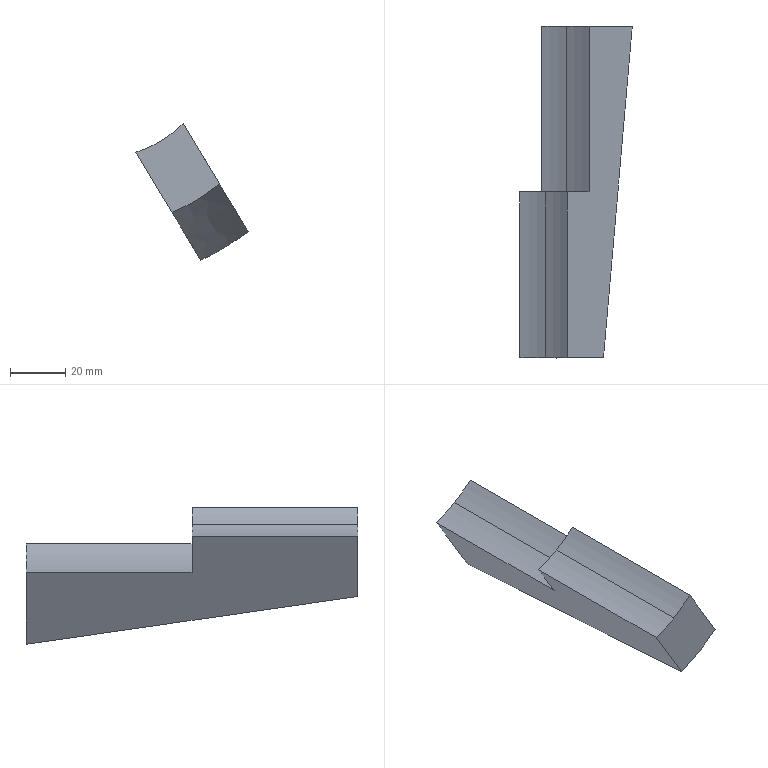Part | STEP file | 2026.6.15-Main Assembly图.sldasm-Part-37 | 1 solid | 10 faces | box 40.625 x 120 x 49.357 mm | volume 66279 mm3 | plane 5 | cylinder 4 | spline 1 | commonest cylinder face diameters 90 x2 120 x2
STEP:
#1=CARTESIAN_POINT('',(-731.198,648.541,3155.98));
#2=VERTEX_POINT('',#1);
#3=CARTESIAN_POINT('',(-740.348,648.541,3151.791));
#4=VERTEX_POINT('',#3);
#5=CARTESIAN_POINT('',(-754.391,648.541,3194.543));
#6=DIRECTION('',(0.,1.,0.));
#7=DIRECTION('',(0.5154,0.,-0.8569));
#8=AXIS2_PLACEMENT_3D('',#5,#6,#7);
#9=CIRCLE('',#8,45.);
#10=EDGE_CURVE('',#2,#4,#9,.T.);
#11=ORIENTED_EDGE('',*,*,#10,.F.);
#12=CARTESIAN_POINT('',(-731.198,708.541,3155.98));
#13=VERTEX_POINT('',#12);
#14=CARTESIAN_POINT('',(-731.198,648.541,3155.98));
#15=DIRECTION('',(0.,1.,0.));
#16=VECTOR('',#15,1000.);
#17=LINE('',#14,#16);
#18=EDGE_CURVE('',#2,#13,#17,.T.);
#19=ORIENTED_EDGE('',*,*,#18,.T.);
#20=CARTESIAN_POINT('',(-740.348,708.541,3151.791));
#21=VERTEX_POINT('',#20);
#22=CARTESIAN_POINT('',(-754.391,708.541,3194.543));
#23=DIRECTION('',(0.,-1.,0.));
#24=DIRECTION('',(0.5154,0.,-0.8569));
#25=AXIS2_PLACEMENT_3D('',#22,#23,#24);
#26=CIRCLE('',#25,45.);
#27=EDGE_CURVE('',#21,#13,#26,.T.);
#28=ORIENTED_EDGE('',*,*,#27,.F.);
#29=CARTESIAN_POINT('',(-740.348,648.541,3151.791));
#30=DIRECTION('',(0.,-1.,0.));
#31=VECTOR('',#30,1000.);
#32=LINE('',#29,#31);
#33=EDGE_CURVE('',#21,#4,#32,.T.);
#34=ORIENTED_EDGE('',*,*,#33,.T.);
#35=EDGE_LOOP('',(#11,#19,#28,#34));
#36=FACE_OUTER_BOUND('',#35,.T.);
#37=CARTESIAN_POINT('',(-754.391,648.541,3194.543));
#38=DIRECTION('',(0.,1.,0.));
#39=DIRECTION('',(-0.5154,0.,0.8569));
#40=AXIS2_PLACEMENT_3D('',#37,#38,#39);
#41=CYLINDRICAL_SURFACE('',#40,45.);
#42=ADVANCED_FACE('',(#36),#41,.F.);
#43=CARTESIAN_POINT('',(-723.467,708.541,3143.126));
#44=VERTEX_POINT('',#43);
#45=CARTESIAN_POINT('',(-732.469,708.541,3138.691));
#46=VERTEX_POINT('',#45);
#47=CARTESIAN_POINT('',(-754.391,708.541,3194.543));
#48=DIRECTION('',(0.,1.,0.));
#49=DIRECTION('',(0.5154,0.,-0.8569));
#50=AXIS2_PLACEMENT_3D('',#47,#48,#49);
#51=CIRCLE('',#50,60.);
#52=EDGE_CURVE('',#44,#46,#51,.T.);
#53=ORIENTED_EDGE('',*,*,#52,.F.);
#54=CARTESIAN_POINT('',(-723.467,768.541,3143.126));
#55=VERTEX_POINT('',#54);
#56=CARTESIAN_POINT('',(-723.467,708.541,3143.126));
#57=DIRECTION('',(0.,1.,0.));
#58=VECTOR('',#57,1000.);
#59=LINE('',#56,#58);
#60=EDGE_CURVE('',#44,#55,#59,.T.);
#61=ORIENTED_EDGE('',*,*,#60,.T.);
#62=CARTESIAN_POINT('',(-732.469,768.541,3138.691));
#63=VERTEX_POINT('',#62);
#64=CARTESIAN_POINT('',(-754.391,768.541,3194.543));
#65=DIRECTION('',(0.,1.,0.));
#66=DIRECTION('',(0.5154,0.,-0.8569));
#67=AXIS2_PLACEMENT_3D('',#64,#65,#66);
#68=CIRCLE('',#67,60.);
#69=EDGE_CURVE('',#55,#63,#68,.T.);
#70=ORIENTED_EDGE('',*,*,#69,.T.);
#71=CARTESIAN_POINT('',(-732.469,708.541,3138.691));
#72=DIRECTION('',(0.,-1.,0.));
#73=VECTOR('',#72,1000.);
#74=LINE('',#71,#73);
#75=EDGE_CURVE('',#63,#46,#74,.T.);
#76=ORIENTED_EDGE('',*,*,#75,.T.);
#77=EDGE_LOOP('',(#53,#61,#70,#76));
#78=FACE_OUTER_BOUND('',#77,.T.);
#79=CARTESIAN_POINT('',(-754.391,708.541,3194.543));
#80=DIRECTION('',(0.,1.,0.));
#81=DIRECTION('',(-0.5154,0.,0.8569));
#82=AXIS2_PLACEMENT_3D('',#79,#80,#81);
#83=CYLINDRICAL_SURFACE('',#82,60.);
#84=ADVANCED_FACE('',(#78),#83,.F.);
#85=ORIENTED_EDGE('',*,*,#60,.F.);
#86=CARTESIAN_POINT('',(-715.33,708.541,3148.999));
#87=VERTEX_POINT('',#86);
#88=CARTESIAN_POINT('',(-754.391,708.541,3194.543));
#89=DIRECTION('',(0.,1.,0.));
#90=DIRECTION('',(0.5154,0.,-0.8569));
#91=AXIS2_PLACEMENT_3D('',#88,#89,#90);
#92=CIRCLE('',#91,60.);
#93=EDGE_CURVE('',#87,#44,#92,.T.);
#94=ORIENTED_EDGE('',*,*,#93,.F.);
#95=CARTESIAN_POINT('',(-715.33,768.541,3148.999));
#96=VERTEX_POINT('',#95);
#97=CARTESIAN_POINT('',(-715.33,708.541,3148.999));
#98=DIRECTION('',(0.,1.,0.));
#99=VECTOR('',#98,1000.);
#100=LINE('',#97,#99);
#101=EDGE_CURVE('',#87,#96,#100,.T.);
#102=ORIENTED_EDGE('',*,*,#101,.T.);
#103=CARTESIAN_POINT('',(-754.391,768.541,3194.543));
#104=DIRECTION('',(0.,1.,0.));
#105=DIRECTION('',(0.5154,0.,-0.8569));
#106=AXIS2_PLACEMENT_3D('',#103,#104,#105);
#107=CIRCLE('',#106,60.);
#108=EDGE_CURVE('',#96,#55,#107,.T.);
#109=ORIENTED_EDGE('',*,*,#108,.T.);
#110=EDGE_LOOP('',(#85,#94,#102,#109));
#111=FACE_OUTER_BOUND('',#110,.T.);
#112=CARTESIAN_POINT('',(-754.391,708.541,3194.543));
#113=DIRECTION('',(0.,1.,0.));
#114=DIRECTION('',(-0.5154,0.,0.8569));
#115=AXIS2_PLACEMENT_3D('',#112,#113,#114);
#116=CYLINDRICAL_SURFACE('',#115,60.);
#117=ADVANCED_FACE('',(#111),#116,.F.);
#118=CARTESIAN_POINT('',(-723.209,708.541,3162.099));
#119=VERTEX_POINT('',#118);
#120=CARTESIAN_POINT('',(-745.822,708.541,3199.697));
#121=DIRECTION('',(-0.5154,0.,0.8569));
#122=VECTOR('',#121,1000.);
#123=LINE('',#120,#122);
#124=EDGE_CURVE('',#87,#119,#123,.T.);
#125=ORIENTED_EDGE('',*,*,#124,.F.);
#126=ORIENTED_EDGE('',*,*,#93,.T.);
#127=ORIENTED_EDGE('',*,*,#52,.T.);
#128=CARTESIAN_POINT('',(-762.961,708.541,3189.389));
#129=DIRECTION('',(0.5154,0.,-0.8569));
#130=VECTOR('',#129,1000.);
#131=LINE('',#128,#130);
#132=EDGE_CURVE('',#21,#46,#131,.T.);
#133=ORIENTED_EDGE('',*,*,#132,.F.);
#134=ORIENTED_EDGE('',*,*,#27,.T.);
#135=CARTESIAN_POINT('',(-754.391,708.541,3194.543));
#136=DIRECTION('',(0.,-1.,0.));
#137=DIRECTION('',(0.5154,0.,-0.8569));
#138=AXIS2_PLACEMENT_3D('',#135,#136,#137);
#139=CIRCLE('',#138,45.);
#140=EDGE_CURVE('',#13,#119,#139,.T.);
#141=ORIENTED_EDGE('',*,*,#140,.T.);
#142=EDGE_LOOP('',(#125,#126,#127,#133,#134,#141));
#143=FACE_OUTER_BOUND('',#142,.T.);
#144=CARTESIAN_POINT('',(-754.391,708.541,3194.543));
#145=DIRECTION('',(0.,1.,0.));
#146=DIRECTION('',(0.8569,0.,0.5154));
#147=AXIS2_PLACEMENT_3D('',#144,#145,#146);
#148=PLANE('',#147);
#149=ADVANCED_FACE('',(#143),#148,.T.);
#150=CARTESIAN_POINT('',(-710.114,648.541,3140.326));
#151=VERTEX_POINT('',#150);
#152=CARTESIAN_POINT('',(-699.723,768.541,3123.049));
#153=VERTEX_POINT('',#152);
#154=CARTESIAN_POINT('',(-710.114,648.541,3140.326));
#155=CARTESIAN_POINT('',(-709.101,660.212,3138.642));
#156=CARTESIAN_POINT('',(-708.089,671.882,3136.959));
#157=CARTESIAN_POINT('',(-707.077,683.553,3135.278));
#158=CARTESIAN_POINT('',(-706.066,695.224,3133.596));
#159=CARTESIAN_POINT('',(-705.055,706.895,3131.916));
#160=CARTESIAN_POINT('',(-704.045,718.566,3130.236));
#161=CARTESIAN_POINT('',(-702.603,735.224,3127.839));
#162=CARTESIAN_POINT('',(-701.163,751.882,3125.443));
#163=CARTESIAN_POINT('',(-699.723,768.541,3123.049));
#164=B_SPLINE_CURVE_WITH_KNOTS('',3,(#154,#155,#156,#157,#158,#159,#160,#161,#162,#163),.UNSPECIFIED.,.F.,.F.,(4,3,3,4),(0.,0.0355,0.07101,0.1217),.UNSPECIFIED.);
#165=EDGE_CURVE('',#151,#153,#164,.T.);
#166=ORIENTED_EDGE('',*,*,#165,.F.);
#167=CARTESIAN_POINT('',(-727.253,648.541,3130.018));
#168=VERTEX_POINT('',#167);
#169=CARTESIAN_POINT('',(-710.114,648.541,3140.326));
#170=CARTESIAN_POINT('',(-712.704,648.541,3138.21));
#171=CARTESIAN_POINT('',(-718.189,648.541,3134.35));
#172=CARTESIAN_POINT('',(-724.17,648.541,3131.315));
#173=CARTESIAN_POINT('',(-727.253,648.541,3130.018));
#174=B_SPLINE_CURVE_WITH_KNOTS('',3,(#169,#170,#171,#172,#173),.UNSPECIFIED.,.F.,.F.,(4,1,4),(0.,0.01,0.02),.UNSPECIFIED.);
#175=EDGE_CURVE('',#151,#168,#174,.T.);
#176=ORIENTED_EDGE('',*,*,#175,.T.);
#177=CARTESIAN_POINT('',(-716.862,768.541,3112.741));
#178=VERTEX_POINT('',#177);
#179=CARTESIAN_POINT('',(-716.862,768.541,3112.741));
#180=CARTESIAN_POINT('',(-717.925,756.246,3114.508));
#181=CARTESIAN_POINT('',(-718.988,743.952,3116.276));
#182=CARTESIAN_POINT('',(-720.051,731.657,3118.045));
#183=CARTESIAN_POINT('',(-721.115,719.363,3119.813));
#184=CARTESIAN_POINT('',(-722.179,707.068,3121.583));
#185=CARTESIAN_POINT('',(-723.244,694.774,3123.353));
#186=CARTESIAN_POINT('',(-724.579,679.363,3125.573));
#187=CARTESIAN_POINT('',(-725.915,663.952,3127.794));
#188=CARTESIAN_POINT('',(-727.253,648.541,3130.018));
#189=B_SPLINE_CURVE_WITH_KNOTS('',3,(#179,#180,#181,#182,#183,#184,#185,#186,#187,#188),.UNSPECIFIED.,.F.,.F.,(4,3,3,4),(0.,0.0374,0.0748,0.1217),.UNSPECIFIED.);
#190=EDGE_CURVE('',#178,#168,#189,.T.);
#191=ORIENTED_EDGE('',*,*,#190,.F.);
#192=CARTESIAN_POINT('',(-699.723,768.541,3123.049));
#193=CARTESIAN_POINT('',(-702.376,768.541,3121.02));
#194=CARTESIAN_POINT('',(-707.909,768.541,3117.258));
#195=CARTESIAN_POINT('',(-713.826,768.541,3114.134));
#196=CARTESIAN_POINT('',(-716.862,768.541,3112.741));
#197=B_SPLINE_CURVE_WITH_KNOTS('',3,(#192,#193,#194,#195,#196),.UNSPECIFIED.,.F.,.F.,(4,1,4),(0.,0.01,0.02),.UNSPECIFIED.);
#198=EDGE_CURVE('',#153,#178,#197,.T.);
#199=ORIENTED_EDGE('',*,*,#198,.F.);
#200=EDGE_LOOP('',(#166,#176,#191,#199));
#201=FACE_OUTER_BOUND('',#200,.T.);
#202=CARTESIAN_POINT('',(-677.094,769.741,3241.032));
#203=CARTESIAN_POINT('',(-677.152,769.341,3240.998));
#204=CARTESIAN_POINT('',(-677.209,768.941,3240.964));
#205=CARTESIAN_POINT('',(-677.266,768.541,3240.929));
#206=CARTESIAN_POINT('',(-682.979,728.541,3237.493));
#207=CARTESIAN_POINT('',(-688.692,688.541,3234.057));
#208=CARTESIAN_POINT('',(-694.405,648.541,3230.621));
#209=CARTESIAN_POINT('',(-680.137,769.741,3246.091));
#210=CARTESIAN_POINT('',(-680.192,769.341,3246.053));
#211=CARTESIAN_POINT('',(-680.247,768.941,3246.015));
#212=CARTESIAN_POINT('',(-680.302,768.541,3245.977));
#213=CARTESIAN_POINT('',(-685.79,728.541,3242.167));
#214=CARTESIAN_POINT('',(-691.278,688.541,3238.357));
#215=CARTESIAN_POINT('',(-696.766,648.541,3234.547));
#216=CARTESIAN_POINT('',(-687.219,769.741,3255.61));
#217=CARTESIAN_POINT('',(-687.268,769.341,3255.565));
#218=CARTESIAN_POINT('',(-687.318,768.941,3255.52));
#219=CARTESIAN_POINT('',(-687.368,768.541,3255.475));
#220=CARTESIAN_POINT('',(-692.332,728.541,3250.961));
#221=CARTESIAN_POINT('',(-697.297,688.541,3246.448));
#222=CARTESIAN_POINT('',(-702.262,648.541,3241.934));
#223=CARTESIAN_POINT('',(-700.423,769.741,3267.541));
#224=CARTESIAN_POINT('',(-700.463,769.341,3267.487));
#225=CARTESIAN_POINT('',(-700.503,768.941,3267.433));
#226=CARTESIAN_POINT('',(-700.543,768.541,3267.379));
#227=CARTESIAN_POINT('',(-704.532,728.541,3261.984));
#228=CARTESIAN_POINT('',(-708.52,688.541,3256.589));
#229=CARTESIAN_POINT('',(-712.509,648.541,3251.194));
#230=CARTESIAN_POINT('',(-715.701,769.741,3276.667));
#231=CARTESIAN_POINT('',(-715.73,769.341,3276.607));
#232=CARTESIAN_POINT('',(-715.759,768.941,3276.546));
#233=CARTESIAN_POINT('',(-715.787,768.541,3276.485));
#234=CARTESIAN_POINT('',(-718.647,728.541,3270.415));
#235=CARTESIAN_POINT('',(-721.506,688.541,3264.346));
#236=CARTESIAN_POINT('',(-724.366,648.541,3258.276));
#237=CARTESIAN_POINT('',(-732.467,769.741,3282.637));
#238=CARTESIAN_POINT('',(-732.483,769.341,3282.572));
#239=CARTESIAN_POINT('',(-732.499,768.941,3282.507));
#240=CARTESIAN_POINT('',(-732.515,768.541,3282.442));
#241=CARTESIAN_POINT('',(-734.136,728.541,3275.931));
#242=CARTESIAN_POINT('',(-735.756,688.541,3269.42));
#243=CARTESIAN_POINT('',(-737.376,648.541,3262.909));
#244=CARTESIAN_POINT('',(-750.074,769.741,3285.222));
#245=CARTESIAN_POINT('',(-750.077,769.341,3285.155));
#246=CARTESIAN_POINT('',(-750.08,768.941,3285.088));
#247=CARTESIAN_POINT('',(-750.084,768.541,3285.021));
#248=CARTESIAN_POINT('',(-750.403,728.541,3278.319));
#249=CARTESIAN_POINT('',(-750.722,688.541,3271.617));
#250=CARTESIAN_POINT('',(-751.041,648.541,3264.915));
#251=CARTESIAN_POINT('',(-767.848,769.741,3284.322));
#252=CARTESIAN_POINT('',(-767.838,769.341,3284.255));
#253=CARTESIAN_POINT('',(-767.828,768.941,3284.189));
#254=CARTESIAN_POINT('',(-767.818,768.541,3284.123));
#255=CARTESIAN_POINT('',(-766.823,728.541,3277.487));
#256=CARTESIAN_POINT('',(-765.829,688.541,3270.852));
#257=CARTESIAN_POINT('',(-764.834,648.541,3264.216));
#258=CARTESIAN_POINT('',(-785.104,769.741,3279.971));
#259=CARTESIAN_POINT('',(-785.081,769.341,3279.908));
#260=CARTESIAN_POINT('',(-785.059,768.941,3279.845));
#261=CARTESIAN_POINT('',(-785.036,768.541,3279.782));
#262=CARTESIAN_POINT('',(-782.766,728.541,3273.468));
#263=CARTESIAN_POINT('',(-780.496,688.541,3267.154));
#264=CARTESIAN_POINT('',(-778.226,648.541,3260.84));
#265=CARTESIAN_POINT('',(-801.18,769.741,3272.338));
#266=CARTESIAN_POINT('',(-801.146,769.341,3272.281));
#267=CARTESIAN_POINT('',(-801.111,768.941,3272.223));
#268=CARTESIAN_POINT('',(-801.076,768.541,3272.166));
#269=CARTESIAN_POINT('',(-797.618,728.541,3266.416));
#270=CARTESIAN_POINT('',(-794.16,688.541,3260.666));
#271=CARTESIAN_POINT('',(-790.702,648.541,3254.916));
#272=CARTESIAN_POINT('',(-815.458,769.741,3261.715));
#273=CARTESIAN_POINT('',(-815.413,769.341,3261.666));
#274=CARTESIAN_POINT('',(-815.368,768.941,3261.616));
#275=CARTESIAN_POINT('',(-815.323,768.541,3261.566));
#276=CARTESIAN_POINT('',(-810.809,728.541,3256.602));
#277=CARTESIAN_POINT('',(-806.296,688.541,3251.637));
#278=CARTESIAN_POINT('',(-801.783,648.541,3246.672));
#279=CARTESIAN_POINT('',(-827.39,769.741,3248.511));
#280=CARTESIAN_POINT('',(-827.336,769.341,3248.471));
#281=CARTESIAN_POINT('',(-827.282,768.941,3248.431));
#282=CARTESIAN_POINT('',(-827.228,768.541,3248.391));
#283=CARTESIAN_POINT('',(-821.832,728.541,3244.403));
#284=CARTESIAN_POINT('',(-816.437,688.541,3240.414));
#285=CARTESIAN_POINT('',(-811.042,648.541,3236.425));
#286=CARTESIAN_POINT('',(-836.516,769.741,3233.233));
#287=CARTESIAN_POINT('',(-836.455,769.341,3233.204));
#288=CARTESIAN_POINT('',(-836.394,768.941,3233.176));
#289=CARTESIAN_POINT('',(-836.333,768.541,3233.147));
#290=CARTESIAN_POINT('',(-830.264,728.541,3230.287));
#291=CARTESIAN_POINT('',(-824.194,688.541,3227.428));
#292=CARTESIAN_POINT('',(-818.124,648.541,3224.568));
#293=CARTESIAN_POINT('',(-842.486,769.741,3216.468));
#294=CARTESIAN_POINT('',(-842.42,769.341,3216.451));
#295=CARTESIAN_POINT('',(-842.355,768.941,3216.435));
#296=CARTESIAN_POINT('',(-842.29,768.541,3216.419));
#297=CARTESIAN_POINT('',(-835.779,728.541,3214.799));
#298=CARTESIAN_POINT('',(-829.268,688.541,3213.178));
#299=CARTESIAN_POINT('',(-822.757,648.541,3211.558));
#300=CARTESIAN_POINT('',(-845.07,769.741,3198.86));
#301=CARTESIAN_POINT('',(-845.003,769.341,3198.857));
#302=CARTESIAN_POINT('',(-844.936,768.941,3198.854));
#303=CARTESIAN_POINT('',(-844.869,768.541,3198.85));
#304=CARTESIAN_POINT('',(-838.167,728.541,3198.531));
#305=CARTESIAN_POINT('',(-831.465,688.541,3198.212));
#306=CARTESIAN_POINT('',(-824.763,648.541,3197.893));
#307=CARTESIAN_POINT('',(-844.17,769.741,3181.087));
#308=CARTESIAN_POINT('',(-844.104,769.341,3181.097));
#309=CARTESIAN_POINT('',(-844.037,768.941,3181.106));
#310=CARTESIAN_POINT('',(-843.971,768.541,3181.116));
#311=CARTESIAN_POINT('',(-837.335,728.541,3182.111));
#312=CARTESIAN_POINT('',(-830.7,688.541,3183.106));
#313=CARTESIAN_POINT('',(-824.064,648.541,3184.1));
#314=CARTESIAN_POINT('',(-839.82,769.741,3163.83));
#315=CARTESIAN_POINT('',(-839.757,769.341,3163.853));
#316=CARTESIAN_POINT('',(-839.694,768.941,3163.875));
#317=CARTESIAN_POINT('',(-839.63,768.541,3163.898));
#318=CARTESIAN_POINT('',(-833.316,728.541,3166.168));
#319=CARTESIAN_POINT('',(-827.002,688.541,3168.438));
#320=CARTESIAN_POINT('',(-820.688,648.541,3170.708));
#321=CARTESIAN_POINT('',(-834.731,769.741,3153.113));
#322=CARTESIAN_POINT('',(-834.671,769.341,3153.143));
#323=CARTESIAN_POINT('',(-834.612,768.941,3153.174));
#324=CARTESIAN_POINT('',(-834.553,768.541,3153.205));
#325=CARTESIAN_POINT('',(-828.615,728.541,3156.267));
#326=CARTESIAN_POINT('',(-822.677,688.541,3159.329));
#327=CARTESIAN_POINT('',(-816.739,648.541,3162.391));
#328=CARTESIAN_POINT('',(-828.645,769.741,3142.995));
#329=CARTESIAN_POINT('',(-828.59,769.341,3143.033));
#330=CARTESIAN_POINT('',(-828.535,768.941,3143.071));
#331=CARTESIAN_POINT('',(-828.481,768.541,3143.109));
#332=CARTESIAN_POINT('',(-822.993,728.541,3146.919));
#333=CARTESIAN_POINT('',(-817.504,688.541,3150.729));
#334=CARTESIAN_POINT('',(-812.016,648.541,3154.539));
#335=CARTESIAN_POINT('',(-821.564,769.741,3133.476));
#336=CARTESIAN_POINT('',(-821.514,769.341,3133.521));
#337=CARTESIAN_POINT('',(-821.464,768.941,3133.566));
#338=CARTESIAN_POINT('',(-821.415,768.541,3133.611));
#339=CARTESIAN_POINT('',(-816.45,728.541,3138.125));
#340=CARTESIAN_POINT('',(-811.485,688.541,3142.638));
#341=CARTESIAN_POINT('',(-806.521,648.541,3147.152));
#342=CARTESIAN_POINT('',(-808.359,769.741,3121.545));
#343=CARTESIAN_POINT('',(-808.319,769.341,3121.599));
#344=CARTESIAN_POINT('',(-808.279,768.941,3121.653));
#345=CARTESIAN_POINT('',(-808.239,768.541,3121.707));
#346=CARTESIAN_POINT('',(-804.251,728.541,3127.102));
#347=CARTESIAN_POINT('',(-800.262,688.541,3132.497));
#348=CARTESIAN_POINT('',(-796.273,648.541,3137.892));
#349=CARTESIAN_POINT('',(-793.081,769.741,3112.419));
#350=CARTESIAN_POINT('',(-793.052,769.341,3112.479));
#351=CARTESIAN_POINT('',(-793.024,768.941,3112.54));
#352=CARTESIAN_POINT('',(-792.995,768.541,3112.601));
#353=CARTESIAN_POINT('',(-790.136,728.541,3118.671));
#354=CARTESIAN_POINT('',(-787.276,688.541,3124.74));
#355=CARTESIAN_POINT('',(-784.417,648.541,3130.81));
#356=CARTESIAN_POINT('',(-776.316,769.741,3106.449));
#357=CARTESIAN_POINT('',(-776.3,769.341,3106.514));
#358=CARTESIAN_POINT('',(-776.283,768.941,3106.579));
#359=CARTESIAN_POINT('',(-776.267,768.541,3106.644));
#360=CARTESIAN_POINT('',(-774.647,728.541,3113.155));
#361=CARTESIAN_POINT('',(-773.026,688.541,3119.666));
#362=CARTESIAN_POINT('',(-771.406,648.541,3126.177));
#363=CARTESIAN_POINT('',(-758.708,769.741,3103.864));
#364=CARTESIAN_POINT('',(-758.705,769.341,3103.931));
#365=CARTESIAN_POINT('',(-758.702,768.941,3103.998));
#366=CARTESIAN_POINT('',(-758.699,768.541,3104.065));
#367=CARTESIAN_POINT('',(-758.38,728.541,3110.767));
#368=CARTESIAN_POINT('',(-758.061,688.541,3117.469));
#369=CARTESIAN_POINT('',(-757.741,648.541,3124.171));
#370=CARTESIAN_POINT('',(-740.935,769.741,3104.764));
#371=CARTESIAN_POINT('',(-740.945,769.341,3104.831));
#372=CARTESIAN_POINT('',(-740.955,768.941,3104.897));
#373=CARTESIAN_POINT('',(-740.965,768.541,3104.963));
#374=CARTESIAN_POINT('',(-741.959,728.541,3111.599));
#375=CARTESIAN_POINT('',(-742.954,688.541,3118.234));
#376=CARTESIAN_POINT('',(-743.948,648.541,3124.87));
#377=CARTESIAN_POINT('',(-723.678,769.741,3109.115));
#378=CARTESIAN_POINT('',(-723.701,769.341,3109.178));
#379=CARTESIAN_POINT('',(-723.724,768.941,3109.241));
#380=CARTESIAN_POINT('',(-723.746,768.541,3109.304));
#381=CARTESIAN_POINT('',(-726.016,728.541,3115.618));
#382=CARTESIAN_POINT('',(-728.286,688.541,3121.932));
#383=CARTESIAN_POINT('',(-730.556,648.541,3128.246));
#384=CARTESIAN_POINT('',(-707.602,769.741,3116.748));
#385=CARTESIAN_POINT('',(-707.637,769.341,3116.805));
#386=CARTESIAN_POINT('',(-707.671,768.941,3116.863));
#387=CARTESIAN_POINT('',(-707.706,768.541,3116.92));
#388=CARTESIAN_POINT('',(-711.164,728.541,3122.67));
#389=CARTESIAN_POINT('',(-714.622,688.541,3128.42));
#390=CARTESIAN_POINT('',(-718.08,648.541,3134.17));
#391=CARTESIAN_POINT('',(-693.324,769.741,3127.371));
#392=CARTESIAN_POINT('',(-693.369,769.341,3127.42));
#393=CARTESIAN_POINT('',(-693.414,768.941,3127.47));
#394=CARTESIAN_POINT('',(-693.46,768.541,3127.52));
#395=CARTESIAN_POINT('',(-697.973,728.541,3132.484));
#396=CARTESIAN_POINT('',(-702.486,688.541,3137.449));
#397=CARTESIAN_POINT('',(-707.,648.541,3142.414));
#398=CARTESIAN_POINT('',(-681.393,769.741,3140.575));
#399=CARTESIAN_POINT('',(-681.447,769.341,3140.615));
#400=CARTESIAN_POINT('',(-681.501,768.941,3140.655));
#401=CARTESIAN_POINT('',(-681.555,768.541,3140.695));
#402=CARTESIAN_POINT('',(-686.95,728.541,3144.683));
#403=CARTESIAN_POINT('',(-692.345,688.541,3148.672));
#404=CARTESIAN_POINT('',(-697.741,648.541,3152.661));
#405=CARTESIAN_POINT('',(-672.267,769.741,3155.853));
#406=CARTESIAN_POINT('',(-672.328,769.341,3155.882));
#407=CARTESIAN_POINT('',(-672.388,768.941,3155.91));
#408=CARTESIAN_POINT('',(-672.449,768.541,3155.939));
#409=CARTESIAN_POINT('',(-678.519,728.541,3158.799));
#410=CARTESIAN_POINT('',(-684.589,688.541,3161.658));
#411=CARTESIAN_POINT('',(-690.658,648.541,3164.518));
#412=CARTESIAN_POINT('',(-666.297,769.741,3172.618));
#413=CARTESIAN_POINT('',(-666.362,769.341,3172.635));
#414=CARTESIAN_POINT('',(-666.427,768.941,3172.651));
#415=CARTESIAN_POINT('',(-666.492,768.541,3172.667));
#416=CARTESIAN_POINT('',(-673.003,728.541,3174.287));
#417=CARTESIAN_POINT('',(-679.514,688.541,3175.908));
#418=CARTESIAN_POINT('',(-686.025,648.541,3177.528));
#419=CARTESIAN_POINT('',(-663.712,769.741,3190.226));
#420=CARTESIAN_POINT('',(-663.779,769.341,3190.229));
#421=CARTESIAN_POINT('',(-663.846,768.941,3190.232));
#422=CARTESIAN_POINT('',(-663.913,768.541,3190.236));
#423=CARTESIAN_POINT('',(-670.615,728.541,3190.555));
#424=CARTESIAN_POINT('',(-677.317,688.541,3190.874));
#425=CARTESIAN_POINT('',(-684.02,648.541,3191.193));
#426=CARTESIAN_POINT('',(-664.612,769.741,3207.999));
#427=CARTESIAN_POINT('',(-664.679,769.341,3207.99));
#428=CARTESIAN_POINT('',(-664.745,768.941,3207.98));
#429=CARTESIAN_POINT('',(-664.812,768.541,3207.97));
#430=CARTESIAN_POINT('',(-671.447,728.541,3206.975));
#431=CARTESIAN_POINT('',(-678.083,688.541,3205.981));
#432=CARTESIAN_POINT('',(-684.718,648.541,3204.986));
#433=CARTESIAN_POINT('',(-668.963,769.741,3225.256));
#434=CARTESIAN_POINT('',(-669.026,769.341,3225.233));
#435=CARTESIAN_POINT('',(-669.089,768.941,3225.211));
#436=CARTESIAN_POINT('',(-669.152,768.541,3225.188));
#437=CARTESIAN_POINT('',(-675.466,728.541,3222.918));
#438=CARTESIAN_POINT('',(-681.78,688.541,3220.648));
#439=CARTESIAN_POINT('',(-688.094,648.541,3218.378));
#440=CARTESIAN_POINT('',(-674.052,769.741,3235.973));
#441=CARTESIAN_POINT('',(-674.111,769.341,3235.943));
#442=CARTESIAN_POINT('',(-674.17,768.941,3235.912));
#443=CARTESIAN_POINT('',(-674.23,768.541,3235.881));
#444=CARTESIAN_POINT('',(-680.168,728.541,3232.819));
#445=CARTESIAN_POINT('',(-686.106,688.541,3229.757));
#446=CARTESIAN_POINT('',(-692.043,648.541,3226.695));
#447=CARTESIAN_POINT('',(-677.094,769.741,3241.032));
#448=CARTESIAN_POINT('',(-677.152,769.341,3240.998));
#449=CARTESIAN_POINT('',(-677.209,768.941,3240.964));
#450=CARTESIAN_POINT('',(-677.266,768.541,3240.929));
#451=CARTESIAN_POINT('',(-682.979,728.541,3237.493));
#452=CARTESIAN_POINT('',(-688.692,688.541,3234.057));
#453=CARTESIAN_POINT('',(-694.405,648.541,3230.621));
#454=B_SPLINE_SURFACE_WITH_KNOTS('',3,3,((#202,#203,#204,#205,#206,#207,#208),(#209,#210,#211,#212,#213,#214,#215),(#216,#217,#218,#219,#220,#221,#222),(#223,#224,#225,#226,#227,#228,#229),(#230,#231,#232,#233,#234,#235,#236),(#237,#238,#239,#240,#241,#242,#243),(#244,#245,#246,#247,#248,#249,#250),(#251,#252,#253,#254,#255,#256,#257),(#258,#259,#260,#261,#262,#263,#264),(#265,#266,#267,#268,#269,#270,#271),(#272,#273,#274,#275,#276,#277,#278),(#279,#280,#281,#282,#283,#284,#285),(#286,#287,#288,#289,#290,#291,#292),(#293,#294,#295,#296,#297,#298,#299),(#300,#301,#302,#303,#304,#305,#306),(#307,#308,#309,#310,#311,#312,#313),(#314,#315,#316,#317,#318,#319,#320),(#321,#322,#323,#324,#325,#326,#327),(#328,#329,#330,#331,#332,#333,#334),(#335,#336,#337,#338,#339,#340,#341),(#342,#343,#344,#345,#346,#347,#348),(#349,#350,#351,#352,#353,#354,#355),(#356,#357,#358,#359,#360,#361,#362),(#363,#364,#365,#366,#367,#368,#369),(#370,#371,#372,#373,#374,#375,#376),(#377,#378,#379,#380,#381,#382,#383),(#384,#385,#386,#387,#388,#389,#390),(#391,#392,#393,#394,#395,#396,#397),(#398,#399,#400,#401,#402,#403,#404),(#405,#406,#407,#408,#409,#410,#411),(#412,#413,#414,#415,#416,#417,#418),(#419,#420,#421,#422,#423,#424,#425),(#426,#427,#428,#429,#430,#431,#432),(#433,#434,#435,#436,#437,#438,#439),(#440,#441,#442,#443,#444,#445,#446),(#447,#448,#449,#450,#451,#452,#453)),.UNSPECIFIED.,.T.,.F.,.F.,(4,1,1,1,1,1,1,1,1,1,1,1,1,1,1,1,2,1,1,1,1,1,1,1,1,1,1,1,1,1,1,1,4),(4,3,4),(0.,0.03125,0.0625,0.09375,0.125,0.1562,0.1875,0.2188,0.25,0.2812,0.3125,0.3438,0.375,0.4062,0.4375,0.4688,0.5,0.5312,0.5625,0.5938,0.625,0.6562,0.6875,0.7188,0.75,0.7812,0.8125,0.8438,0.875,0.9062,0.9375,0.9688,1.),(-0.01,0.,1.),.UNSPECIFIED.);
#455=ADVANCED_FACE('',(#201),#454,.T.);
#456=CARTESIAN_POINT('',(-742.846,768.541,3194.749));
#457=DIRECTION('',(-0.5154,0.,0.8569));
#458=VECTOR('',#457,1000.);
#459=LINE('',#456,#458);
#460=EDGE_CURVE('',#153,#96,#459,.T.);
#461=ORIENTED_EDGE('',*,*,#460,.F.);
#462=ORIENTED_EDGE('',*,*,#198,.T.);
#463=CARTESIAN_POINT('',(-759.985,768.541,3184.441));
#464=DIRECTION('',(0.5154,0.,-0.8569));
#465=VECTOR('',#464,1000.);
#466=LINE('',#463,#465);
#467=EDGE_CURVE('',#63,#178,#466,.T.);
#468=ORIENTED_EDGE('',*,*,#467,.F.);
#469=ORIENTED_EDGE('',*,*,#69,.F.);
#470=ORIENTED_EDGE('',*,*,#108,.F.);
#471=EDGE_LOOP('',(#461,#462,#468,#469,#470));
#472=FACE_OUTER_BOUND('',#471,.T.);
#473=CARTESIAN_POINT('',(-754.391,768.541,3194.543));
#474=DIRECTION('',(0.,1.,0.));
#475=DIRECTION('',(0.8569,0.,0.5154));
#476=AXIS2_PLACEMENT_3D('',#473,#474,#475);
#477=PLANE('',#476);
#478=ADVANCED_FACE('',(#472),#477,.T.);
#479=ORIENTED_EDGE('',*,*,#175,.F.);
#480=CARTESIAN_POINT('',(-723.209,648.541,3162.099));
#481=VERTEX_POINT('',#480);
#482=CARTESIAN_POINT('',(-742.846,648.541,3194.749));
#483=DIRECTION('',(-0.5154,0.,0.8569));
#484=VECTOR('',#483,1000.);
#485=LINE('',#482,#484);
#486=EDGE_CURVE('',#151,#481,#485,.T.);
#487=ORIENTED_EDGE('',*,*,#486,.T.);
#488=CARTESIAN_POINT('',(-754.391,648.541,3194.543));
#489=DIRECTION('',(0.,1.,0.));
#490=DIRECTION('',(0.5154,0.,-0.8569));
#491=AXIS2_PLACEMENT_3D('',#488,#489,#490);
#492=CIRCLE('',#491,45.);
#493=EDGE_CURVE('',#481,#2,#492,.T.);
#494=ORIENTED_EDGE('',*,*,#493,.T.);
#495=ORIENTED_EDGE('',*,*,#10,.T.);
#496=CARTESIAN_POINT('',(-759.985,648.541,3184.441));
#497=DIRECTION('',(0.5154,0.,-0.8569));
#498=VECTOR('',#497,1000.);
#499=LINE('',#496,#498);
#500=EDGE_CURVE('',#4,#168,#499,.T.);
#501=ORIENTED_EDGE('',*,*,#500,.T.);
#502=EDGE_LOOP('',(#479,#487,#494,#495,#501));
#503=FACE_OUTER_BOUND('',#502,.T.);
#504=CARTESIAN_POINT('',(-754.391,648.541,3194.543));
#505=DIRECTION('',(0.,1.,0.));
#506=DIRECTION('',(0.8569,0.,0.5154));
#507=AXIS2_PLACEMENT_3D('',#504,#505,#506);
#508=PLANE('',#507);
#509=ADVANCED_FACE('',(#503),#508,.F.);
#510=ORIENTED_EDGE('',*,*,#18,.F.);
#511=ORIENTED_EDGE('',*,*,#493,.F.);
#512=CARTESIAN_POINT('',(-723.209,648.541,3162.099));
#513=DIRECTION('',(0.,1.,0.));
#514=VECTOR('',#513,1000.);
#515=LINE('',#512,#514);
#516=EDGE_CURVE('',#481,#119,#515,.T.);
#517=ORIENTED_EDGE('',*,*,#516,.T.);
#518=ORIENTED_EDGE('',*,*,#140,.F.);
#519=EDGE_LOOP('',(#510,#511,#517,#518));
#520=FACE_OUTER_BOUND('',#519,.T.);
#521=CARTESIAN_POINT('',(-754.391,648.541,3194.543));
#522=DIRECTION('',(0.,1.,0.));
#523=DIRECTION('',(-0.5154,0.,0.8569));
#524=AXIS2_PLACEMENT_3D('',#521,#522,#523);
#525=CYLINDRICAL_SURFACE('',#524,45.);
#526=ADVANCED_FACE('',(#520),#525,.F.);
#527=ORIENTED_EDGE('',*,*,#190,.T.);
#528=ORIENTED_EDGE('',*,*,#500,.F.);
#529=ORIENTED_EDGE('',*,*,#33,.F.);
#530=ORIENTED_EDGE('',*,*,#132,.T.);
#531=ORIENTED_EDGE('',*,*,#75,.F.);
#532=ORIENTED_EDGE('',*,*,#467,.T.);
#533=EDGE_LOOP('',(#527,#528,#529,#530,#531,#532));
#534=FACE_OUTER_BOUND('',#533,.T.);
#535=CARTESIAN_POINT('',(-759.985,648.541,3184.441));
#536=DIRECTION('',(0.8569,0.,0.5154));
#537=DIRECTION('',(-0.5154,0.,0.8569));
#538=AXIS2_PLACEMENT_3D('',#535,#536,#537);
#539=PLANE('',#538);
#540=ADVANCED_FACE('',(#534),#539,.F.);
#541=ORIENTED_EDGE('',*,*,#165,.T.);
#542=ORIENTED_EDGE('',*,*,#460,.T.);
#543=ORIENTED_EDGE('',*,*,#101,.F.);
#544=ORIENTED_EDGE('',*,*,#124,.T.);
#545=ORIENTED_EDGE('',*,*,#516,.F.);
#546=ORIENTED_EDGE('',*,*,#486,.F.);
#547=EDGE_LOOP('',(#541,#542,#543,#544,#545,#546));
#548=FACE_OUTER_BOUND('',#547,.T.);
#549=CARTESIAN_POINT('',(-742.846,648.541,3194.749));
#550=DIRECTION('',(-0.8569,0.,-0.5154));
#551=DIRECTION('',(0.5154,0.,-0.8569));
#552=AXIS2_PLACEMENT_3D('',#549,#550,#551);
#553=PLANE('',#552);
#554=ADVANCED_FACE('',(#548),#553,.F.);
#555=CLOSED_SHELL('',(#42,#84,#117,#149,#455,#478,#509,#526,#540,#554));
#556=MANIFOLD_SOLID_BREP('',#555);
#557=CARTESIAN_POINT('',(0.,0.,0.));
#558=DIRECTION('',(0.,0.,1.));
#559=DIRECTION('',(1.,0.,0.));
#560=AXIS2_PLACEMENT_3D('',#557,#558,#559);
#561=(LENGTH_UNIT()NAMED_UNIT(*)SI_UNIT(.MILLI.,.METRE.));
#562=UNCERTAINTY_MEASURE_WITH_UNIT(LENGTH_MEASURE(0.00001),#561,'','');
#563=(NAMED_UNIT(*)PLANE_ANGLE_UNIT()SI_UNIT($,.RADIAN.));
#564=(NAMED_UNIT(*)SI_UNIT($,.STERADIAN.)SOLID_ANGLE_UNIT());
#565=(GEOMETRIC_REPRESENTATION_CONTEXT(3)GLOBAL_UNCERTAINTY_ASSIGNED_CONTEXT((#562))GLOBAL_UNIT_ASSIGNED_CONTEXT((#561,#563,#564))REPRESENTATION_CONTEXT('',''));
#566=ADVANCED_BREP_SHAPE_REPRESENTATION('',(#556,#560),#565);